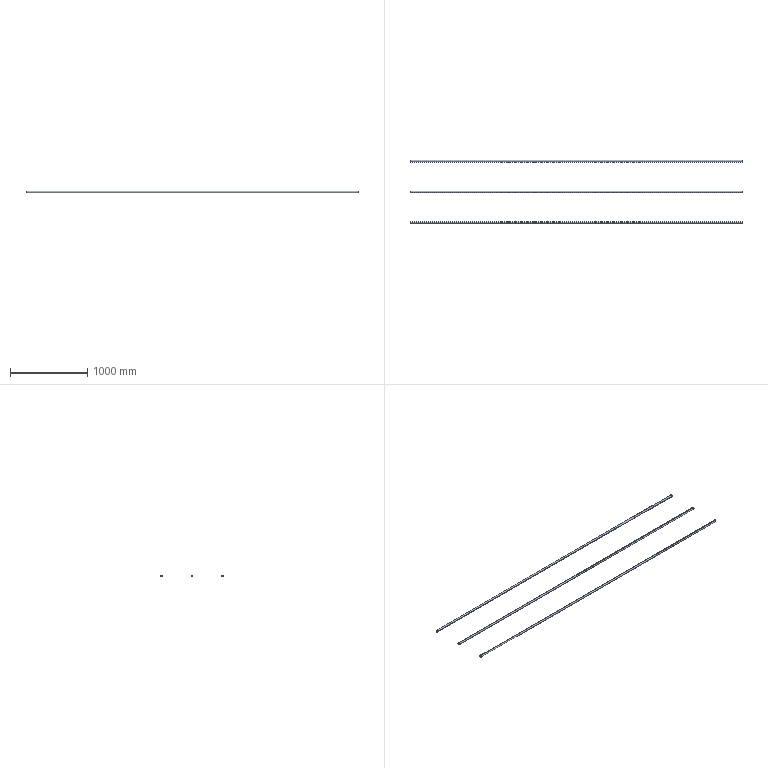Part | STEP file | 粉仓护栏栏杆1_Default<As Machined> | 3 solids | 18 faces | box 4305 x 825 x 25 mm | volume 1430222 mm3 | cylinder 12 | plane 6 | commonest cylinder face diameters 22 x6 25 x6
STEP:
#1=CARTESIAN_POINT('',(0.,0.,0.));
#2=DIRECTION('',(0.,0.,1.));
#3=DIRECTION('',(1.,0.,0.));
#4=AXIS2_PLACEMENT_3D('',#1,#2,#3);
#5=CARTESIAN_POINT('',(-4305.,0.,12.5));
#6=VERTEX_POINT('',#5);
#7=CARTESIAN_POINT('',(-4305.,0.,-12.5));
#8=VERTEX_POINT('',#7);
#9=CARTESIAN_POINT('',(-4305.,0.,0.));
#10=DIRECTION('',(-1.,0.,0.));
#11=DIRECTION('',(0.,-1.,0.));
#12=AXIS2_PLACEMENT_3D('',#9,#10,#11);
#13=CIRCLE('',#12,12.5);
#14=CARTESIAN_POINT('',(-4305.,0.,0.));
#15=DIRECTION('',(1.,0.,0.));
#16=DIRECTION('',(0.,0.,-1.));
#17=AXIS2_PLACEMENT_3D('',#14,#15,#16);
#18=CYLINDRICAL_SURFACE('',#17,12.5);
#19=CARTESIAN_POINT('',(4.712,0.));
#20=DIRECTION('',(-1.,0.));
#21=VECTOR('',#20,1.);
#22=LINE('',#19,#21);
#23=(GEOMETRIC_REPRESENTATION_CONTEXT(2)PARAMETRIC_REPRESENTATION_CONTEXT()REPRESENTATION_CONTEXT('',''));
#24=DEFINITIONAL_REPRESENTATION('',(#22),#23);
#25=PCURVE('',#18,#24);
#26=CARTESIAN_POINT('',(-4305.,0.,0.));
#27=DIRECTION('',(-1.,0.,0.));
#28=DIRECTION('',(0.,-1.,0.));
#29=AXIS2_PLACEMENT_3D('',#26,#27,#28);
#30=PLANE('',#29);
#31=CARTESIAN_POINT('',(0.,0.));
#32=DIRECTION('',(1.,0.));
#33=AXIS2_PLACEMENT_2D('',#31,#32);
#34=CIRCLE('',#33,12.5);
#35=(GEOMETRIC_REPRESENTATION_CONTEXT(2)PARAMETRIC_REPRESENTATION_CONTEXT()REPRESENTATION_CONTEXT('',''));
#36=DEFINITIONAL_REPRESENTATION('',(#34),#35);
#37=PCURVE('',#30,#36);
#38=SURFACE_CURVE('',#13,(#25,#37),.PCURVE_S1.);
#39=EDGE_CURVE('',#6,#8,#38,.T.);
#40=ORIENTED_EDGE('',*,*,#39,.F.);
#41=CARTESIAN_POINT('',(0.,0.,12.5));
#42=VERTEX_POINT('',#41);
#43=CARTESIAN_POINT('',(-4305.,0.,12.5));
#44=DIRECTION('',(1.,0.,0.));
#45=VECTOR('',#44,1.);
#46=LINE('',#43,#45);
#47=CARTESIAN_POINT('',(3.142,0.));
#48=DIRECTION('',(0.,1.));
#49=VECTOR('',#48,1.);
#50=LINE('',#47,#49);
#51=(GEOMETRIC_REPRESENTATION_CONTEXT(2)PARAMETRIC_REPRESENTATION_CONTEXT()REPRESENTATION_CONTEXT('',''));
#52=DEFINITIONAL_REPRESENTATION('',(#50),#51);
#53=PCURVE('',#18,#52);
#54=CARTESIAN_POINT('',(-4305.,0.,0.));
#55=DIRECTION('',(1.,0.,0.));
#56=DIRECTION('',(0.,0.,-1.));
#57=AXIS2_PLACEMENT_3D('',#54,#55,#56);
#58=CYLINDRICAL_SURFACE('',#57,12.5);
#59=CARTESIAN_POINT('',(3.142,0.));
#60=DIRECTION('',(0.,1.));
#61=VECTOR('',#60,1.);
#62=LINE('',#59,#61);
#63=(GEOMETRIC_REPRESENTATION_CONTEXT(2)PARAMETRIC_REPRESENTATION_CONTEXT()REPRESENTATION_CONTEXT('',''));
#64=DEFINITIONAL_REPRESENTATION('',(#62),#63);
#65=PCURVE('',#58,#64);
#66=SURFACE_CURVE('',#46,(#53,#65),.PCURVE_S1.);
#67=EDGE_CURVE('',#6,#42,#66,.T.);
#68=ORIENTED_EDGE('',*,*,#67,.T.);
#69=CARTESIAN_POINT('',(0.,0.,-12.5));
#70=VERTEX_POINT('',#69);
#71=CARTESIAN_POINT('',(0.,0.,0.));
#72=DIRECTION('',(-1.,0.,0.));
#73=DIRECTION('',(0.,-1.,0.));
#74=AXIS2_PLACEMENT_3D('',#71,#72,#73);
#75=CIRCLE('',#74,12.5);
#76=CARTESIAN_POINT('',(4.712,4305.));
#77=DIRECTION('',(-1.,0.));
#78=VECTOR('',#77,1.);
#79=LINE('',#76,#78);
#80=(GEOMETRIC_REPRESENTATION_CONTEXT(2)PARAMETRIC_REPRESENTATION_CONTEXT()REPRESENTATION_CONTEXT('',''));
#81=DEFINITIONAL_REPRESENTATION('',(#79),#80);
#82=PCURVE('',#18,#81);
#83=CARTESIAN_POINT('',(0.,0.,0.));
#84=DIRECTION('',(-1.,0.,0.));
#85=DIRECTION('',(0.,-1.,0.));
#86=AXIS2_PLACEMENT_3D('',#83,#84,#85);
#87=PLANE('',#86);
#88=CARTESIAN_POINT('',(0.,0.));
#89=DIRECTION('',(1.,0.));
#90=AXIS2_PLACEMENT_2D('',#88,#89);
#91=CIRCLE('',#90,12.5);
#92=(GEOMETRIC_REPRESENTATION_CONTEXT(2)PARAMETRIC_REPRESENTATION_CONTEXT()REPRESENTATION_CONTEXT('',''));
#93=DEFINITIONAL_REPRESENTATION('',(#91),#92);
#94=PCURVE('',#87,#93);
#95=SURFACE_CURVE('',#75,(#82,#94),.PCURVE_S1.);
#96=EDGE_CURVE('',#42,#70,#95,.T.);
#97=ORIENTED_EDGE('',*,*,#96,.T.);
#98=CARTESIAN_POINT('',(-4305.,0.,-12.5));
#99=DIRECTION('',(1.,0.,0.));
#100=VECTOR('',#99,1.);
#101=LINE('',#98,#100);
#102=CARTESIAN_POINT('',(0.,0.));
#103=DIRECTION('',(0.,1.));
#104=VECTOR('',#103,1.);
#105=LINE('',#102,#104);
#106=(GEOMETRIC_REPRESENTATION_CONTEXT(2)PARAMETRIC_REPRESENTATION_CONTEXT()REPRESENTATION_CONTEXT('',''));
#107=DEFINITIONAL_REPRESENTATION('',(#105),#106);
#108=PCURVE('',#18,#107);
#109=CARTESIAN_POINT('',(6.283,0.));
#110=DIRECTION('',(0.,1.));
#111=VECTOR('',#110,1.);
#112=LINE('',#109,#111);
#113=(GEOMETRIC_REPRESENTATION_CONTEXT(2)PARAMETRIC_REPRESENTATION_CONTEXT()REPRESENTATION_CONTEXT('',''));
#114=DEFINITIONAL_REPRESENTATION('',(#112),#113);
#115=PCURVE('',#58,#114);
#116=SURFACE_CURVE('',#101,(#108,#115),.PCURVE_S1.);
#117=EDGE_CURVE('',#8,#70,#116,.T.);
#118=ORIENTED_EDGE('',*,*,#117,.F.);
#119=EDGE_LOOP('',(#40,#68,#97,#118));
#120=FACE_BOUND('',#119,.T.);
#121=ADVANCED_FACE('',(#120),#18,.T.);
#122=CARTESIAN_POINT('',(-4305.,0.,-11.));
#123=VERTEX_POINT('',#122);
#124=CARTESIAN_POINT('',(0.,0.,-11.));
#125=VERTEX_POINT('',#124);
#126=CARTESIAN_POINT('',(-4305.,0.,-11.));
#127=DIRECTION('',(1.,0.,0.));
#128=VECTOR('',#127,1.);
#129=LINE('',#126,#128);
#130=CARTESIAN_POINT('',(-4305.,0.,0.));
#131=DIRECTION('',(1.,0.,0.));
#132=DIRECTION('',(0.,0.,-1.));
#133=AXIS2_PLACEMENT_3D('',#130,#131,#132);
#134=CYLINDRICAL_SURFACE('',#133,11.);
#135=CARTESIAN_POINT('',(6.283,0.));
#136=DIRECTION('',(0.,1.));
#137=VECTOR('',#136,1.);
#138=LINE('',#135,#137);
#139=(GEOMETRIC_REPRESENTATION_CONTEXT(2)PARAMETRIC_REPRESENTATION_CONTEXT()REPRESENTATION_CONTEXT('',''));
#140=DEFINITIONAL_REPRESENTATION('',(#138),#139);
#141=PCURVE('',#134,#140);
#142=CARTESIAN_POINT('',(-4305.,0.,0.));
#143=DIRECTION('',(1.,0.,0.));
#144=DIRECTION('',(0.,0.,-1.));
#145=AXIS2_PLACEMENT_3D('',#142,#143,#144);
#146=CYLINDRICAL_SURFACE('',#145,11.);
#147=CARTESIAN_POINT('',(0.,0.));
#148=DIRECTION('',(0.,1.));
#149=VECTOR('',#148,1.);
#150=LINE('',#147,#149);
#151=(GEOMETRIC_REPRESENTATION_CONTEXT(2)PARAMETRIC_REPRESENTATION_CONTEXT()REPRESENTATION_CONTEXT('',''));
#152=DEFINITIONAL_REPRESENTATION('',(#150),#151);
#153=PCURVE('',#146,#152);
#154=SURFACE_CURVE('',#129,(#141,#153),.PCURVE_S1.);
#155=EDGE_CURVE('',#123,#125,#154,.T.);
#156=ORIENTED_EDGE('',*,*,#155,.T.);
#157=CARTESIAN_POINT('',(0.,0.,11.));
#158=VERTEX_POINT('',#157);
#159=CARTESIAN_POINT('',(0.,0.,0.));
#160=DIRECTION('',(-1.,0.,0.));
#161=DIRECTION('',(0.,-1.,0.));
#162=AXIS2_PLACEMENT_3D('',#159,#160,#161);
#163=CIRCLE('',#162,11.);
#164=CARTESIAN_POINT('',(10.996,4305.));
#165=DIRECTION('',(-1.,0.));
#166=VECTOR('',#165,1.);
#167=LINE('',#164,#166);
#168=(GEOMETRIC_REPRESENTATION_CONTEXT(2)PARAMETRIC_REPRESENTATION_CONTEXT()REPRESENTATION_CONTEXT('',''));
#169=DEFINITIONAL_REPRESENTATION('',(#167),#168);
#170=PCURVE('',#134,#169);
#171=CARTESIAN_POINT('',(0.,0.));
#172=DIRECTION('',(1.,0.));
#173=AXIS2_PLACEMENT_2D('',#171,#172);
#174=CIRCLE('',#173,11.);
#175=(GEOMETRIC_REPRESENTATION_CONTEXT(2)PARAMETRIC_REPRESENTATION_CONTEXT()REPRESENTATION_CONTEXT('',''));
#176=DEFINITIONAL_REPRESENTATION('',(#174),#175);
#177=PCURVE('',#87,#176);
#178=SURFACE_CURVE('',#163,(#170,#177),.PCURVE_S1.);
#179=EDGE_CURVE('',#125,#158,#178,.T.);
#180=ORIENTED_EDGE('',*,*,#179,.T.);
#181=CARTESIAN_POINT('',(-4305.,0.,11.));
#182=VERTEX_POINT('',#181);
#183=CARTESIAN_POINT('',(-4305.,0.,11.));
#184=DIRECTION('',(1.,0.,0.));
#185=VECTOR('',#184,1.);
#186=LINE('',#183,#185);
#187=CARTESIAN_POINT('',(3.142,0.));
#188=DIRECTION('',(0.,1.));
#189=VECTOR('',#188,1.);
#190=LINE('',#187,#189);
#191=(GEOMETRIC_REPRESENTATION_CONTEXT(2)PARAMETRIC_REPRESENTATION_CONTEXT()REPRESENTATION_CONTEXT('',''));
#192=DEFINITIONAL_REPRESENTATION('',(#190),#191);
#193=PCURVE('',#134,#192);
#194=CARTESIAN_POINT('',(3.142,0.));
#195=DIRECTION('',(0.,1.));
#196=VECTOR('',#195,1.);
#197=LINE('',#194,#196);
#198=(GEOMETRIC_REPRESENTATION_CONTEXT(2)PARAMETRIC_REPRESENTATION_CONTEXT()REPRESENTATION_CONTEXT('',''));
#199=DEFINITIONAL_REPRESENTATION('',(#197),#198);
#200=PCURVE('',#146,#199);
#201=SURFACE_CURVE('',#186,(#193,#200),.PCURVE_S1.);
#202=EDGE_CURVE('',#182,#158,#201,.T.);
#203=ORIENTED_EDGE('',*,*,#202,.F.);
#204=CARTESIAN_POINT('',(-4305.,0.,0.));
#205=DIRECTION('',(-1.,0.,0.));
#206=DIRECTION('',(0.,-1.,0.));
#207=AXIS2_PLACEMENT_3D('',#204,#205,#206);
#208=CIRCLE('',#207,11.);
#209=CARTESIAN_POINT('',(10.996,0.));
#210=DIRECTION('',(-1.,0.));
#211=VECTOR('',#210,1.);
#212=LINE('',#209,#211);
#213=(GEOMETRIC_REPRESENTATION_CONTEXT(2)PARAMETRIC_REPRESENTATION_CONTEXT()REPRESENTATION_CONTEXT('',''));
#214=DEFINITIONAL_REPRESENTATION('',(#212),#213);
#215=PCURVE('',#134,#214);
#216=CARTESIAN_POINT('',(0.,0.));
#217=DIRECTION('',(1.,0.));
#218=AXIS2_PLACEMENT_2D('',#216,#217);
#219=CIRCLE('',#218,11.);
#220=(GEOMETRIC_REPRESENTATION_CONTEXT(2)PARAMETRIC_REPRESENTATION_CONTEXT()REPRESENTATION_CONTEXT('',''));
#221=DEFINITIONAL_REPRESENTATION('',(#219),#220);
#222=PCURVE('',#30,#221);
#223=SURFACE_CURVE('',#208,(#215,#222),.PCURVE_S1.);
#224=EDGE_CURVE('',#123,#182,#223,.T.);
#225=ORIENTED_EDGE('',*,*,#224,.F.);
#226=EDGE_LOOP('',(#156,#180,#203,#225));
#227=FACE_BOUND('',#226,.F.);
#228=ADVANCED_FACE('',(#227),#134,.F.);
#229=CARTESIAN_POINT('',(0.,0.,0.));
#230=DIRECTION('',(-1.,0.,0.));
#231=DIRECTION('',(0.,-1.,0.));
#232=AXIS2_PLACEMENT_3D('',#229,#230,#231);
#233=CIRCLE('',#232,11.);
#234=CARTESIAN_POINT('',(4.712,4305.));
#235=DIRECTION('',(-1.,0.));
#236=VECTOR('',#235,1.);
#237=LINE('',#234,#236);
#238=(GEOMETRIC_REPRESENTATION_CONTEXT(2)PARAMETRIC_REPRESENTATION_CONTEXT()REPRESENTATION_CONTEXT('',''));
#239=DEFINITIONAL_REPRESENTATION('',(#237),#238);
#240=PCURVE('',#146,#239);
#241=CARTESIAN_POINT('',(0.,0.));
#242=DIRECTION('',(1.,0.));
#243=AXIS2_PLACEMENT_2D('',#241,#242);
#244=CIRCLE('',#243,11.);
#245=(GEOMETRIC_REPRESENTATION_CONTEXT(2)PARAMETRIC_REPRESENTATION_CONTEXT()REPRESENTATION_CONTEXT('',''));
#246=DEFINITIONAL_REPRESENTATION('',(#244),#245);
#247=PCURVE('',#87,#246);
#248=SURFACE_CURVE('',#233,(#240,#247),.PCURVE_S1.);
#249=EDGE_CURVE('',#158,#125,#248,.T.);
#250=ORIENTED_EDGE('',*,*,#249,.T.);
#251=ORIENTED_EDGE('',*,*,#155,.F.);
#252=CARTESIAN_POINT('',(-4305.,0.,0.));
#253=DIRECTION('',(-1.,0.,0.));
#254=DIRECTION('',(0.,-1.,0.));
#255=AXIS2_PLACEMENT_3D('',#252,#253,#254);
#256=CIRCLE('',#255,11.);
#257=CARTESIAN_POINT('',(4.712,0.));
#258=DIRECTION('',(-1.,0.));
#259=VECTOR('',#258,1.);
#260=LINE('',#257,#259);
#261=(GEOMETRIC_REPRESENTATION_CONTEXT(2)PARAMETRIC_REPRESENTATION_CONTEXT()REPRESENTATION_CONTEXT('',''));
#262=DEFINITIONAL_REPRESENTATION('',(#260),#261);
#263=PCURVE('',#146,#262);
#264=CARTESIAN_POINT('',(0.,0.));
#265=DIRECTION('',(1.,0.));
#266=AXIS2_PLACEMENT_2D('',#264,#265);
#267=CIRCLE('',#266,11.);
#268=(GEOMETRIC_REPRESENTATION_CONTEXT(2)PARAMETRIC_REPRESENTATION_CONTEXT()REPRESENTATION_CONTEXT('',''));
#269=DEFINITIONAL_REPRESENTATION('',(#267),#268);
#270=PCURVE('',#30,#269);
#271=SURFACE_CURVE('',#256,(#263,#270),.PCURVE_S1.);
#272=EDGE_CURVE('',#182,#123,#271,.T.);
#273=ORIENTED_EDGE('',*,*,#272,.F.);
#274=ORIENTED_EDGE('',*,*,#202,.T.);
#275=EDGE_LOOP('',(#250,#251,#273,#274));
#276=FACE_BOUND('',#275,.F.);
#277=ADVANCED_FACE('',(#276),#146,.F.);
#278=ORIENTED_EDGE('',*,*,#67,.F.);
#279=CARTESIAN_POINT('',(-4305.,0.,0.));
#280=DIRECTION('',(-1.,0.,0.));
#281=DIRECTION('',(0.,-1.,0.));
#282=AXIS2_PLACEMENT_3D('',#279,#280,#281);
#283=CIRCLE('',#282,12.5);
#284=CARTESIAN_POINT('',(10.996,0.));
#285=DIRECTION('',(-1.,0.));
#286=VECTOR('',#285,1.);
#287=LINE('',#284,#286);
#288=(GEOMETRIC_REPRESENTATION_CONTEXT(2)PARAMETRIC_REPRESENTATION_CONTEXT()REPRESENTATION_CONTEXT('',''));
#289=DEFINITIONAL_REPRESENTATION('',(#287),#288);
#290=PCURVE('',#58,#289);
#291=CARTESIAN_POINT('',(0.,0.));
#292=DIRECTION('',(1.,0.));
#293=AXIS2_PLACEMENT_2D('',#291,#292);
#294=CIRCLE('',#293,12.5);
#295=(GEOMETRIC_REPRESENTATION_CONTEXT(2)PARAMETRIC_REPRESENTATION_CONTEXT()REPRESENTATION_CONTEXT('',''));
#296=DEFINITIONAL_REPRESENTATION('',(#294),#295);
#297=PCURVE('',#30,#296);
#298=SURFACE_CURVE('',#283,(#290,#297),.PCURVE_S1.);
#299=EDGE_CURVE('',#8,#6,#298,.T.);
#300=ORIENTED_EDGE('',*,*,#299,.F.);
#301=ORIENTED_EDGE('',*,*,#117,.T.);
#302=CARTESIAN_POINT('',(0.,0.,0.));
#303=DIRECTION('',(-1.,0.,0.));
#304=DIRECTION('',(0.,-1.,0.));
#305=AXIS2_PLACEMENT_3D('',#302,#303,#304);
#306=CIRCLE('',#305,12.5);
#307=CARTESIAN_POINT('',(10.996,4305.));
#308=DIRECTION('',(-1.,0.));
#309=VECTOR('',#308,1.);
#310=LINE('',#307,#309);
#311=(GEOMETRIC_REPRESENTATION_CONTEXT(2)PARAMETRIC_REPRESENTATION_CONTEXT()REPRESENTATION_CONTEXT('',''));
#312=DEFINITIONAL_REPRESENTATION('',(#310),#311);
#313=PCURVE('',#58,#312);
#314=CARTESIAN_POINT('',(0.,0.));
#315=DIRECTION('',(1.,0.));
#316=AXIS2_PLACEMENT_2D('',#314,#315);
#317=CIRCLE('',#316,12.5);
#318=(GEOMETRIC_REPRESENTATION_CONTEXT(2)PARAMETRIC_REPRESENTATION_CONTEXT()REPRESENTATION_CONTEXT('',''));
#319=DEFINITIONAL_REPRESENTATION('',(#317),#318);
#320=PCURVE('',#87,#319);
#321=SURFACE_CURVE('',#306,(#313,#320),.PCURVE_S1.);
#322=EDGE_CURVE('',#70,#42,#321,.T.);
#323=ORIENTED_EDGE('',*,*,#322,.T.);
#324=EDGE_LOOP('',(#278,#300,#301,#323));
#325=FACE_BOUND('',#324,.T.);
#326=ADVANCED_FACE('',(#325),#58,.T.);
#327=ORIENTED_EDGE('',*,*,#224,.F.);
#328=ORIENTED_EDGE('',*,*,#272,.F.);
#329=EDGE_LOOP('',(#327,#328));
#330=FACE_BOUND('',#329,.T.);
#331=ORIENTED_EDGE('',*,*,#299,.T.);
#332=ORIENTED_EDGE('',*,*,#39,.T.);
#333=EDGE_LOOP('',(#331,#332));
#334=FACE_BOUND('',#333,.T.);
#335=ADVANCED_FACE('',(#330,#334),#30,.T.);
#336=ORIENTED_EDGE('',*,*,#179,.T.);
#337=ORIENTED_EDGE('',*,*,#249,.T.);
#338=EDGE_LOOP('',(#336,#337));
#339=FACE_BOUND('',#338,.T.);
#340=ORIENTED_EDGE('',*,*,#322,.F.);
#341=ORIENTED_EDGE('',*,*,#96,.F.);
#342=EDGE_LOOP('',(#340,#341));
#343=FACE_BOUND('',#342,.T.);
#344=ADVANCED_FACE('',(#339,#343),#87,.F.);
#345=CLOSED_SHELL('',(#121,#228,#277,#326,#335,#344));
#346=MANIFOLD_SOLID_BREP('',#345);
#347=CARTESIAN_POINT('',(-4305.,787.5,0.));
#348=VERTEX_POINT('',#347);
#349=CARTESIAN_POINT('',(-4305.,812.5,0.));
#350=VERTEX_POINT('',#349);
#351=CARTESIAN_POINT('',(-4305.,800.,0.));
#352=DIRECTION('',(-1.,0.,0.));
#353=DIRECTION('',(0.,-1.,0.));
#354=AXIS2_PLACEMENT_3D('',#351,#352,#353);
#355=CIRCLE('',#354,12.5);
#356=CARTESIAN_POINT('',(-4305.,800.,0.));
#357=DIRECTION('',(1.,0.,0.));
#358=DIRECTION('',(0.,1.,0.));
#359=AXIS2_PLACEMENT_3D('',#356,#357,#358);
#360=CYLINDRICAL_SURFACE('',#359,12.5);
#361=CARTESIAN_POINT('',(3.142,0.));
#362=DIRECTION('',(-1.,0.));
#363=VECTOR('',#362,1.);
#364=LINE('',#361,#363);
#365=(GEOMETRIC_REPRESENTATION_CONTEXT(2)PARAMETRIC_REPRESENTATION_CONTEXT()REPRESENTATION_CONTEXT('',''));
#366=DEFINITIONAL_REPRESENTATION('',(#364),#365);
#367=PCURVE('',#360,#366);
#368=CARTESIAN_POINT('',(-4305.,800.,0.));
#369=DIRECTION('',(-1.,0.,0.));
#370=DIRECTION('',(0.,-1.,0.));
#371=AXIS2_PLACEMENT_3D('',#368,#369,#370);
#372=PLANE('',#371);
#373=CARTESIAN_POINT('',(0.,0.));
#374=DIRECTION('',(1.,0.));
#375=AXIS2_PLACEMENT_2D('',#373,#374);
#376=CIRCLE('',#375,12.5);
#377=(GEOMETRIC_REPRESENTATION_CONTEXT(2)PARAMETRIC_REPRESENTATION_CONTEXT()REPRESENTATION_CONTEXT('',''));
#378=DEFINITIONAL_REPRESENTATION('',(#376),#377);
#379=PCURVE('',#372,#378);
#380=SURFACE_CURVE('',#355,(#367,#379),.PCURVE_S1.);
#381=EDGE_CURVE('',#348,#350,#380,.T.);
#382=ORIENTED_EDGE('',*,*,#381,.F.);
#383=CARTESIAN_POINT('',(0.,787.5,0.));
#384=VERTEX_POINT('',#383);
#385=CARTESIAN_POINT('',(-4305.,787.5,0.));
#386=DIRECTION('',(1.,0.,0.));
#387=VECTOR('',#386,1.);
#388=LINE('',#385,#387);
#389=CARTESIAN_POINT('',(3.142,0.));
#390=DIRECTION('',(0.,1.));
#391=VECTOR('',#390,1.);
#392=LINE('',#389,#391);
#393=(GEOMETRIC_REPRESENTATION_CONTEXT(2)PARAMETRIC_REPRESENTATION_CONTEXT()REPRESENTATION_CONTEXT('',''));
#394=DEFINITIONAL_REPRESENTATION('',(#392),#393);
#395=PCURVE('',#360,#394);
#396=CARTESIAN_POINT('',(-4305.,800.,0.));
#397=DIRECTION('',(1.,0.,0.));
#398=DIRECTION('',(0.,1.,0.));
#399=AXIS2_PLACEMENT_3D('',#396,#397,#398);
#400=CYLINDRICAL_SURFACE('',#399,12.5);
#401=CARTESIAN_POINT('',(3.142,0.));
#402=DIRECTION('',(0.,1.));
#403=VECTOR('',#402,1.);
#404=LINE('',#401,#403);
#405=(GEOMETRIC_REPRESENTATION_CONTEXT(2)PARAMETRIC_REPRESENTATION_CONTEXT()REPRESENTATION_CONTEXT('',''));
#406=DEFINITIONAL_REPRESENTATION('',(#404),#405);
#407=PCURVE('',#400,#406);
#408=SURFACE_CURVE('',#388,(#395,#407),.PCURVE_S1.);
#409=EDGE_CURVE('',#348,#384,#408,.T.);
#410=ORIENTED_EDGE('',*,*,#409,.T.);
#411=CARTESIAN_POINT('',(0.,812.5,0.));
#412=VERTEX_POINT('',#411);
#413=CARTESIAN_POINT('',(0.,800.,0.));
#414=DIRECTION('',(-1.,0.,0.));
#415=DIRECTION('',(0.,-1.,0.));
#416=AXIS2_PLACEMENT_3D('',#413,#414,#415);
#417=CIRCLE('',#416,12.5);
#418=CARTESIAN_POINT('',(3.142,4305.));
#419=DIRECTION('',(-1.,0.));
#420=VECTOR('',#419,1.);
#421=LINE('',#418,#420);
#422=(GEOMETRIC_REPRESENTATION_CONTEXT(2)PARAMETRIC_REPRESENTATION_CONTEXT()REPRESENTATION_CONTEXT('',''));
#423=DEFINITIONAL_REPRESENTATION('',(#421),#422);
#424=PCURVE('',#360,#423);
#425=CARTESIAN_POINT('',(0.,800.,0.));
#426=DIRECTION('',(-1.,0.,0.));
#427=DIRECTION('',(0.,-1.,0.));
#428=AXIS2_PLACEMENT_3D('',#425,#426,#427);
#429=PLANE('',#428);
#430=CARTESIAN_POINT('',(0.,0.));
#431=DIRECTION('',(1.,0.));
#432=AXIS2_PLACEMENT_2D('',#430,#431);
#433=CIRCLE('',#432,12.5);
#434=(GEOMETRIC_REPRESENTATION_CONTEXT(2)PARAMETRIC_REPRESENTATION_CONTEXT()REPRESENTATION_CONTEXT('',''));
#435=DEFINITIONAL_REPRESENTATION('',(#433),#434);
#436=PCURVE('',#429,#435);
#437=SURFACE_CURVE('',#417,(#424,#436),.PCURVE_S1.);
#438=EDGE_CURVE('',#384,#412,#437,.T.);
#439=ORIENTED_EDGE('',*,*,#438,.T.);
#440=CARTESIAN_POINT('',(-4305.,812.5,0.));
#441=DIRECTION('',(1.,0.,0.));
#442=VECTOR('',#441,1.);
#443=LINE('',#440,#442);
#444=CARTESIAN_POINT('',(0.,0.));
#445=DIRECTION('',(0.,1.));
#446=VECTOR('',#445,1.);
#447=LINE('',#444,#446);
#448=(GEOMETRIC_REPRESENTATION_CONTEXT(2)PARAMETRIC_REPRESENTATION_CONTEXT()REPRESENTATION_CONTEXT('',''));
#449=DEFINITIONAL_REPRESENTATION('',(#447),#448);
#450=PCURVE('',#360,#449);
#451=CARTESIAN_POINT('',(6.283,0.));
#452=DIRECTION('',(0.,1.));
#453=VECTOR('',#452,1.);
#454=LINE('',#451,#453);
#455=(GEOMETRIC_REPRESENTATION_CONTEXT(2)PARAMETRIC_REPRESENTATION_CONTEXT()REPRESENTATION_CONTEXT('',''));
#456=DEFINITIONAL_REPRESENTATION('',(#454),#455);
#457=PCURVE('',#400,#456);
#458=SURFACE_CURVE('',#443,(#450,#457),.PCURVE_S1.);
#459=EDGE_CURVE('',#350,#412,#458,.T.);
#460=ORIENTED_EDGE('',*,*,#459,.F.);
#461=EDGE_LOOP('',(#382,#410,#439,#460));
#462=FACE_BOUND('',#461,.T.);
#463=ADVANCED_FACE('',(#462),#360,.T.);
#464=CARTESIAN_POINT('',(-4305.,811.,0.));
#465=VERTEX_POINT('',#464);
#466=CARTESIAN_POINT('',(0.,811.,0.));
#467=VERTEX_POINT('',#466);
#468=CARTESIAN_POINT('',(-4305.,811.,0.));
#469=DIRECTION('',(1.,0.,0.));
#470=VECTOR('',#469,1.);
#471=LINE('',#468,#470);
#472=CARTESIAN_POINT('',(-4305.,800.,0.));
#473=DIRECTION('',(1.,0.,0.));
#474=DIRECTION('',(0.,1.,0.));
#475=AXIS2_PLACEMENT_3D('',#472,#473,#474);
#476=CYLINDRICAL_SURFACE('',#475,11.);
#477=CARTESIAN_POINT('',(6.283,0.));
#478=DIRECTION('',(0.,1.));
#479=VECTOR('',#478,1.);
#480=LINE('',#477,#479);
#481=(GEOMETRIC_REPRESENTATION_CONTEXT(2)PARAMETRIC_REPRESENTATION_CONTEXT()REPRESENTATION_CONTEXT('',''));
#482=DEFINITIONAL_REPRESENTATION('',(#480),#481);
#483=PCURVE('',#476,#482);
#484=CARTESIAN_POINT('',(-4305.,800.,0.));
#485=DIRECTION('',(1.,0.,0.));
#486=DIRECTION('',(0.,1.,0.));
#487=AXIS2_PLACEMENT_3D('',#484,#485,#486);
#488=CYLINDRICAL_SURFACE('',#487,11.);
#489=CARTESIAN_POINT('',(0.,0.));
#490=DIRECTION('',(0.,1.));
#491=VECTOR('',#490,1.);
#492=LINE('',#489,#491);
#493=(GEOMETRIC_REPRESENTATION_CONTEXT(2)PARAMETRIC_REPRESENTATION_CONTEXT()REPRESENTATION_CONTEXT('',''));
#494=DEFINITIONAL_REPRESENTATION('',(#492),#493);
#495=PCURVE('',#488,#494);
#496=SURFACE_CURVE('',#471,(#483,#495),.PCURVE_S1.);
#497=EDGE_CURVE('',#465,#467,#496,.T.);
#498=ORIENTED_EDGE('',*,*,#497,.T.);
#499=CARTESIAN_POINT('',(0.,789.,0.));
#500=VERTEX_POINT('',#499);
#501=CARTESIAN_POINT('',(0.,800.,0.));
#502=DIRECTION('',(-1.,0.,0.));
#503=DIRECTION('',(0.,-1.,0.));
#504=AXIS2_PLACEMENT_3D('',#501,#502,#503);
#505=CIRCLE('',#504,11.);
#506=CARTESIAN_POINT('',(9.425,4305.));
#507=DIRECTION('',(-1.,0.));
#508=VECTOR('',#507,1.);
#509=LINE('',#506,#508);
#510=(GEOMETRIC_REPRESENTATION_CONTEXT(2)PARAMETRIC_REPRESENTATION_CONTEXT()REPRESENTATION_CONTEXT('',''));
#511=DEFINITIONAL_REPRESENTATION('',(#509),#510);
#512=PCURVE('',#476,#511);
#513=CARTESIAN_POINT('',(0.,0.));
#514=DIRECTION('',(1.,0.));
#515=AXIS2_PLACEMENT_2D('',#513,#514);
#516=CIRCLE('',#515,11.);
#517=(GEOMETRIC_REPRESENTATION_CONTEXT(2)PARAMETRIC_REPRESENTATION_CONTEXT()REPRESENTATION_CONTEXT('',''));
#518=DEFINITIONAL_REPRESENTATION('',(#516),#517);
#519=PCURVE('',#429,#518);
#520=SURFACE_CURVE('',#505,(#512,#519),.PCURVE_S1.);
#521=EDGE_CURVE('',#467,#500,#520,.T.);
#522=ORIENTED_EDGE('',*,*,#521,.T.);
#523=CARTESIAN_POINT('',(-4305.,789.,0.));
#524=VERTEX_POINT('',#523);
#525=CARTESIAN_POINT('',(-4305.,789.,0.));
#526=DIRECTION('',(1.,0.,0.));
#527=VECTOR('',#526,1.);
#528=LINE('',#525,#527);
#529=CARTESIAN_POINT('',(3.142,0.));
#530=DIRECTION('',(0.,1.));
#531=VECTOR('',#530,1.);
#532=LINE('',#529,#531);
#533=(GEOMETRIC_REPRESENTATION_CONTEXT(2)PARAMETRIC_REPRESENTATION_CONTEXT()REPRESENTATION_CONTEXT('',''));
#534=DEFINITIONAL_REPRESENTATION('',(#532),#533);
#535=PCURVE('',#476,#534);
#536=CARTESIAN_POINT('',(3.142,0.));
#537=DIRECTION('',(0.,1.));
#538=VECTOR('',#537,1.);
#539=LINE('',#536,#538);
#540=(GEOMETRIC_REPRESENTATION_CONTEXT(2)PARAMETRIC_REPRESENTATION_CONTEXT()REPRESENTATION_CONTEXT('',''));
#541=DEFINITIONAL_REPRESENTATION('',(#539),#540);
#542=PCURVE('',#488,#541);
#543=SURFACE_CURVE('',#528,(#535,#542),.PCURVE_S1.);
#544=EDGE_CURVE('',#524,#500,#543,.T.);
#545=ORIENTED_EDGE('',*,*,#544,.F.);
#546=CARTESIAN_POINT('',(-4305.,800.,0.));
#547=DIRECTION('',(-1.,0.,0.));
#548=DIRECTION('',(0.,-1.,0.));
#549=AXIS2_PLACEMENT_3D('',#546,#547,#548);
#550=CIRCLE('',#549,11.);
#551=CARTESIAN_POINT('',(9.425,0.));
#552=DIRECTION('',(-1.,0.));
#553=VECTOR('',#552,1.);
#554=LINE('',#551,#553);
#555=(GEOMETRIC_REPRESENTATION_CONTEXT(2)PARAMETRIC_REPRESENTATION_CONTEXT()REPRESENTATION_CONTEXT('',''));
#556=DEFINITIONAL_REPRESENTATION('',(#554),#555);
#557=PCURVE('',#476,#556);
#558=CARTESIAN_POINT('',(0.,0.));
#559=DIRECTION('',(1.,0.));
#560=AXIS2_PLACEMENT_2D('',#558,#559);
#561=CIRCLE('',#560,11.);
#562=(GEOMETRIC_REPRESENTATION_CONTEXT(2)PARAMETRIC_REPRESENTATION_CONTEXT()REPRESENTATION_CONTEXT('',''));
#563=DEFINITIONAL_REPRESENTATION('',(#561),#562);
#564=PCURVE('',#372,#563);
#565=SURFACE_CURVE('',#550,(#557,#564),.PCURVE_S1.);
#566=EDGE_CURVE('',#465,#524,#565,.T.);
#567=ORIENTED_EDGE('',*,*,#566,.F.);
#568=EDGE_LOOP('',(#498,#522,#545,#567));
#569=FACE_BOUND('',#568,.F.);
#570=ADVANCED_FACE('',(#569),#476,.F.);
#571=CARTESIAN_POINT('',(0.,800.,0.));
#572=DIRECTION('',(-1.,0.,0.));
#573=DIRECTION('',(0.,-1.,0.));
#574=AXIS2_PLACEMENT_3D('',#571,#572,#573);
#575=CIRCLE('',#574,11.);
#576=CARTESIAN_POINT('',(3.142,4305.));
#577=DIRECTION('',(-1.,0.));
#578=VECTOR('',#577,1.);
#579=LINE('',#576,#578);
#580=(GEOMETRIC_REPRESENTATION_CONTEXT(2)PARAMETRIC_REPRESENTATION_CONTEXT()REPRESENTATION_CONTEXT('',''));
#581=DEFINITIONAL_REPRESENTATION('',(#579),#580);
#582=PCURVE('',#488,#581);
#583=CARTESIAN_POINT('',(0.,0.));
#584=DIRECTION('',(1.,0.));
#585=AXIS2_PLACEMENT_2D('',#583,#584);
#586=CIRCLE('',#585,11.);
#587=(GEOMETRIC_REPRESENTATION_CONTEXT(2)PARAMETRIC_REPRESENTATION_CONTEXT()REPRESENTATION_CONTEXT('',''));
#588=DEFINITIONAL_REPRESENTATION('',(#586),#587);
#589=PCURVE('',#429,#588);
#590=SURFACE_CURVE('',#575,(#582,#589),.PCURVE_S1.);
#591=EDGE_CURVE('',#500,#467,#590,.T.);
#592=ORIENTED_EDGE('',*,*,#591,.T.);
#593=ORIENTED_EDGE('',*,*,#497,.F.);
#594=CARTESIAN_POINT('',(-4305.,800.,0.));
#595=DIRECTION('',(-1.,0.,0.));
#596=DIRECTION('',(0.,-1.,0.));
#597=AXIS2_PLACEMENT_3D('',#594,#595,#596);
#598=CIRCLE('',#597,11.);
#599=CARTESIAN_POINT('',(3.142,0.));
#600=DIRECTION('',(-1.,0.));
#601=VECTOR('',#600,1.);
#602=LINE('',#599,#601);
#603=(GEOMETRIC_REPRESENTATION_CONTEXT(2)PARAMETRIC_REPRESENTATION_CONTEXT()REPRESENTATION_CONTEXT('',''));
#604=DEFINITIONAL_REPRESENTATION('',(#602),#603);
#605=PCURVE('',#488,#604);
#606=CARTESIAN_POINT('',(0.,0.));
#607=DIRECTION('',(1.,0.));
#608=AXIS2_PLACEMENT_2D('',#606,#607);
#609=CIRCLE('',#608,11.);
#610=(GEOMETRIC_REPRESENTATION_CONTEXT(2)PARAMETRIC_REPRESENTATION_CONTEXT()REPRESENTATION_CONTEXT('',''));
#611=DEFINITIONAL_REPRESENTATION('',(#609),#610);
#612=PCURVE('',#372,#611);
#613=SURFACE_CURVE('',#598,(#605,#612),.PCURVE_S1.);
#614=EDGE_CURVE('',#524,#465,#613,.T.);
#615=ORIENTED_EDGE('',*,*,#614,.F.);
#616=ORIENTED_EDGE('',*,*,#544,.T.);
#617=EDGE_LOOP('',(#592,#593,#615,#616));
#618=FACE_BOUND('',#617,.F.);
#619=ADVANCED_FACE('',(#618),#488,.F.);
#620=ORIENTED_EDGE('',*,*,#409,.F.);
#621=CARTESIAN_POINT('',(-4305.,800.,0.));
#622=DIRECTION('',(-1.,0.,0.));
#623=DIRECTION('',(0.,-1.,0.));
#624=AXIS2_PLACEMENT_3D('',#621,#622,#623);
#625=CIRCLE('',#624,12.5);
#626=CARTESIAN_POINT('',(9.425,0.));
#627=DIRECTION('',(-1.,0.));
#628=VECTOR('',#627,1.);
#629=LINE('',#626,#628);
#630=(GEOMETRIC_REPRESENTATION_CONTEXT(2)PARAMETRIC_REPRESENTATION_CONTEXT()REPRESENTATION_CONTEXT('',''));
#631=DEFINITIONAL_REPRESENTATION('',(#629),#630);
#632=PCURVE('',#400,#631);
#633=CARTESIAN_POINT('',(0.,0.));
#634=DIRECTION('',(1.,0.));
#635=AXIS2_PLACEMENT_2D('',#633,#634);
#636=CIRCLE('',#635,12.5);
#637=(GEOMETRIC_REPRESENTATION_CONTEXT(2)PARAMETRIC_REPRESENTATION_CONTEXT()REPRESENTATION_CONTEXT('',''));
#638=DEFINITIONAL_REPRESENTATION('',(#636),#637);
#639=PCURVE('',#372,#638);
#640=SURFACE_CURVE('',#625,(#632,#639),.PCURVE_S1.);
#641=EDGE_CURVE('',#350,#348,#640,.T.);
#642=ORIENTED_EDGE('',*,*,#641,.F.);
#643=ORIENTED_EDGE('',*,*,#459,.T.);
#644=CARTESIAN_POINT('',(0.,800.,0.));
#645=DIRECTION('',(-1.,0.,0.));
#646=DIRECTION('',(0.,-1.,0.));
#647=AXIS2_PLACEMENT_3D('',#644,#645,#646);
#648=CIRCLE('',#647,12.5);
#649=CARTESIAN_POINT('',(9.425,4305.));
#650=DIRECTION('',(-1.,0.));
#651=VECTOR('',#650,1.);
#652=LINE('',#649,#651);
#653=(GEOMETRIC_REPRESENTATION_CONTEXT(2)PARAMETRIC_REPRESENTATION_CONTEXT()REPRESENTATION_CONTEXT('',''));
#654=DEFINITIONAL_REPRESENTATION('',(#652),#653);
#655=PCURVE('',#400,#654);
#656=CARTESIAN_POINT('',(0.,0.));
#657=DIRECTION('',(1.,0.));
#658=AXIS2_PLACEMENT_2D('',#656,#657);
#659=CIRCLE('',#658,12.5);
#660=(GEOMETRIC_REPRESENTATION_CONTEXT(2)PARAMETRIC_REPRESENTATION_CONTEXT()REPRESENTATION_CONTEXT('',''));
#661=DEFINITIONAL_REPRESENTATION('',(#659),#660);
#662=PCURVE('',#429,#661);
#663=SURFACE_CURVE('',#648,(#655,#662),.PCURVE_S1.);
#664=EDGE_CURVE('',#412,#384,#663,.T.);
#665=ORIENTED_EDGE('',*,*,#664,.T.);
#666=EDGE_LOOP('',(#620,#642,#643,#665));
#667=FACE_BOUND('',#666,.T.);
#668=ADVANCED_FACE('',(#667),#400,.T.);
#669=ORIENTED_EDGE('',*,*,#566,.F.);
#670=ORIENTED_EDGE('',*,*,#614,.F.);
#671=EDGE_LOOP('',(#669,#670));
#672=FACE_BOUND('',#671,.T.);
#673=ORIENTED_EDGE('',*,*,#641,.T.);
#674=ORIENTED_EDGE('',*,*,#381,.T.);
#675=EDGE_LOOP('',(#673,#674));
#676=FACE_BOUND('',#675,.T.);
#677=ADVANCED_FACE('',(#672,#676),#372,.T.);
#678=ORIENTED_EDGE('',*,*,#521,.T.);
#679=ORIENTED_EDGE('',*,*,#591,.T.);
#680=EDGE_LOOP('',(#678,#679));
#681=FACE_BOUND('',#680,.T.);
#682=ORIENTED_EDGE('',*,*,#664,.F.);
#683=ORIENTED_EDGE('',*,*,#438,.F.);
#684=EDGE_LOOP('',(#682,#683));
#685=FACE_BOUND('',#684,.T.);
#686=ADVANCED_FACE('',(#681,#685),#429,.F.);
#687=CLOSED_SHELL('',(#463,#570,#619,#668,#677,#686));
#688=MANIFOLD_SOLID_BREP('',#687);
#689=CARTESIAN_POINT('',(0.,400.,-12.5));
#690=VERTEX_POINT('',#689);
#691=CARTESIAN_POINT('',(0.,400.,12.5));
#692=VERTEX_POINT('',#691);
#693=CARTESIAN_POINT('',(0.,400.,0.));
#694=DIRECTION('',(1.,0.,0.));
#695=DIRECTION('',(0.,1.,0.));
#696=AXIS2_PLACEMENT_3D('',#693,#694,#695);
#697=CIRCLE('',#696,12.5);
#698=CARTESIAN_POINT('',(0.,400.,0.));
#699=DIRECTION('',(-1.,0.,0.));
#700=DIRECTION('',(0.,0.,1.));
#701=AXIS2_PLACEMENT_3D('',#698,#699,#700);
#702=CYLINDRICAL_SURFACE('',#701,12.5);
#703=CARTESIAN_POINT('',(7.854,0.));
#704=DIRECTION('',(-1.,0.));
#705=VECTOR('',#704,1.);
#706=LINE('',#703,#705);
#707=(GEOMETRIC_REPRESENTATION_CONTEXT(2)PARAMETRIC_REPRESENTATION_CONTEXT()REPRESENTATION_CONTEXT('',''));
#708=DEFINITIONAL_REPRESENTATION('',(#706),#707);
#709=PCURVE('',#702,#708);
#710=CARTESIAN_POINT('',(0.,400.,0.));
#711=DIRECTION('',(1.,0.,0.));
#712=DIRECTION('',(0.,1.,0.));
#713=AXIS2_PLACEMENT_3D('',#710,#711,#712);
#714=PLANE('',#713);
#715=CARTESIAN_POINT('',(0.,0.));
#716=DIRECTION('',(1.,0.));
#717=AXIS2_PLACEMENT_2D('',#715,#716);
#718=CIRCLE('',#717,12.5);
#719=(GEOMETRIC_REPRESENTATION_CONTEXT(2)PARAMETRIC_REPRESENTATION_CONTEXT()REPRESENTATION_CONTEXT('',''));
#720=DEFINITIONAL_REPRESENTATION('',(#718),#719);
#721=PCURVE('',#714,#720);
#722=SURFACE_CURVE('',#697,(#709,#721),.PCURVE_S1.);
#723=EDGE_CURVE('',#690,#692,#722,.T.);
#724=ORIENTED_EDGE('',*,*,#723,.F.);
#725=CARTESIAN_POINT('',(-4305.,400.,-12.5));
#726=VERTEX_POINT('',#725);
#727=CARTESIAN_POINT('',(0.,400.,-12.5));
#728=DIRECTION('',(-1.,0.,0.));
#729=VECTOR('',#728,1.);
#730=LINE('',#727,#729);
#731=CARTESIAN_POINT('',(3.142,0.));
#732=DIRECTION('',(0.,1.));
#733=VECTOR('',#732,1.);
#734=LINE('',#731,#733);
#735=(GEOMETRIC_REPRESENTATION_CONTEXT(2)PARAMETRIC_REPRESENTATION_CONTEXT()REPRESENTATION_CONTEXT('',''));
#736=DEFINITIONAL_REPRESENTATION('',(#734),#735);
#737=PCURVE('',#702,#736);
#738=CARTESIAN_POINT('',(0.,400.,0.));
#739=DIRECTION('',(-1.,0.,0.));
#740=DIRECTION('',(0.,0.,1.));
#741=AXIS2_PLACEMENT_3D('',#738,#739,#740);
#742=CYLINDRICAL_SURFACE('',#741,12.5);
#743=CARTESIAN_POINT('',(3.142,0.));
#744=DIRECTION('',(0.,1.));
#745=VECTOR('',#744,1.);
#746=LINE('',#743,#745);
#747=(GEOMETRIC_REPRESENTATION_CONTEXT(2)PARAMETRIC_REPRESENTATION_CONTEXT()REPRESENTATION_CONTEXT('',''));
#748=DEFINITIONAL_REPRESENTATION('',(#746),#747);
#749=PCURVE('',#742,#748);
#750=SURFACE_CURVE('',#730,(#737,#749),.PCURVE_S1.);
#751=EDGE_CURVE('',#690,#726,#750,.T.);
#752=ORIENTED_EDGE('',*,*,#751,.T.);
#753=CARTESIAN_POINT('',(-4305.,400.,12.5));
#754=VERTEX_POINT('',#753);
#755=CARTESIAN_POINT('',(-4305.,400.,0.));
#756=DIRECTION('',(1.,0.,0.));
#757=DIRECTION('',(0.,1.,0.));
#758=AXIS2_PLACEMENT_3D('',#755,#756,#757);
#759=CIRCLE('',#758,12.5);
#760=CARTESIAN_POINT('',(7.854,4305.));
#761=DIRECTION('',(-1.,0.));
#762=VECTOR('',#761,1.);
#763=LINE('',#760,#762);
#764=(GEOMETRIC_REPRESENTATION_CONTEXT(2)PARAMETRIC_REPRESENTATION_CONTEXT()REPRESENTATION_CONTEXT('',''));
#765=DEFINITIONAL_REPRESENTATION('',(#763),#764);
#766=PCURVE('',#702,#765);
#767=CARTESIAN_POINT('',(-4305.,400.,0.));
#768=DIRECTION('',(1.,0.,0.));
#769=DIRECTION('',(0.,1.,0.));
#770=AXIS2_PLACEMENT_3D('',#767,#768,#769);
#771=PLANE('',#770);
#772=CARTESIAN_POINT('',(0.,0.));
#773=DIRECTION('',(1.,0.));
#774=AXIS2_PLACEMENT_2D('',#772,#773);
#775=CIRCLE('',#774,12.5);
#776=(GEOMETRIC_REPRESENTATION_CONTEXT(2)PARAMETRIC_REPRESENTATION_CONTEXT()REPRESENTATION_CONTEXT('',''));
#777=DEFINITIONAL_REPRESENTATION('',(#775),#776);
#778=PCURVE('',#771,#777);
#779=SURFACE_CURVE('',#759,(#766,#778),.PCURVE_S1.);
#780=EDGE_CURVE('',#726,#754,#779,.T.);
#781=ORIENTED_EDGE('',*,*,#780,.T.);
#782=CARTESIAN_POINT('',(0.,400.,12.5));
#783=DIRECTION('',(-1.,0.,0.));
#784=VECTOR('',#783,1.);
#785=LINE('',#782,#784);
#786=CARTESIAN_POINT('',(0.,0.));
#787=DIRECTION('',(0.,1.));
#788=VECTOR('',#787,1.);
#789=LINE('',#786,#788);
#790=(GEOMETRIC_REPRESENTATION_CONTEXT(2)PARAMETRIC_REPRESENTATION_CONTEXT()REPRESENTATION_CONTEXT('',''));
#791=DEFINITIONAL_REPRESENTATION('',(#789),#790);
#792=PCURVE('',#702,#791);
#793=CARTESIAN_POINT('',(6.283,0.));
#794=DIRECTION('',(0.,1.));
#795=VECTOR('',#794,1.);
#796=LINE('',#793,#795);
#797=(GEOMETRIC_REPRESENTATION_CONTEXT(2)PARAMETRIC_REPRESENTATION_CONTEXT()REPRESENTATION_CONTEXT('',''));
#798=DEFINITIONAL_REPRESENTATION('',(#796),#797);
#799=PCURVE('',#742,#798);
#800=SURFACE_CURVE('',#785,(#792,#799),.PCURVE_S1.);
#801=EDGE_CURVE('',#692,#754,#800,.T.);
#802=ORIENTED_EDGE('',*,*,#801,.F.);
#803=EDGE_LOOP('',(#724,#752,#781,#802));
#804=FACE_BOUND('',#803,.T.);
#805=ADVANCED_FACE('',(#804),#702,.T.);
#806=CARTESIAN_POINT('',(0.,400.,11.));
#807=VERTEX_POINT('',#806);
#808=CARTESIAN_POINT('',(-4305.,400.,11.));
#809=VERTEX_POINT('',#808);
#810=CARTESIAN_POINT('',(0.,400.,11.));
#811=DIRECTION('',(-1.,0.,0.));
#812=VECTOR('',#811,1.);
#813=LINE('',#810,#812);
#814=CARTESIAN_POINT('',(0.,400.,0.));
#815=DIRECTION('',(-1.,0.,0.));
#816=DIRECTION('',(0.,0.,1.));
#817=AXIS2_PLACEMENT_3D('',#814,#815,#816);
#818=CYLINDRICAL_SURFACE('',#817,11.);
#819=CARTESIAN_POINT('',(6.283,0.));
#820=DIRECTION('',(0.,1.));
#821=VECTOR('',#820,1.);
#822=LINE('',#819,#821);
#823=(GEOMETRIC_REPRESENTATION_CONTEXT(2)PARAMETRIC_REPRESENTATION_CONTEXT()REPRESENTATION_CONTEXT('',''));
#824=DEFINITIONAL_REPRESENTATION('',(#822),#823);
#825=PCURVE('',#818,#824);
#826=CARTESIAN_POINT('',(0.,400.,0.));
#827=DIRECTION('',(-1.,0.,0.));
#828=DIRECTION('',(0.,0.,1.));
#829=AXIS2_PLACEMENT_3D('',#826,#827,#828);
#830=CYLINDRICAL_SURFACE('',#829,11.);
#831=CARTESIAN_POINT('',(0.,0.));
#832=DIRECTION('',(0.,1.));
#833=VECTOR('',#832,1.);
#834=LINE('',#831,#833);
#835=(GEOMETRIC_REPRESENTATION_CONTEXT(2)PARAMETRIC_REPRESENTATION_CONTEXT()REPRESENTATION_CONTEXT('',''));
#836=DEFINITIONAL_REPRESENTATION('',(#834),#835);
#837=PCURVE('',#830,#836);
#838=SURFACE_CURVE('',#813,(#825,#837),.PCURVE_S1.);
#839=EDGE_CURVE('',#807,#809,#838,.T.);
#840=ORIENTED_EDGE('',*,*,#839,.T.);
#841=CARTESIAN_POINT('',(-4305.,400.,-11.));
#842=VERTEX_POINT('',#841);
#843=CARTESIAN_POINT('',(-4305.,400.,0.));
#844=DIRECTION('',(1.,0.,0.));
#845=DIRECTION('',(0.,1.,0.));
#846=AXIS2_PLACEMENT_3D('',#843,#844,#845);
#847=CIRCLE('',#846,11.);
#848=CARTESIAN_POINT('',(7.854,4305.));
#849=DIRECTION('',(-1.,0.));
#850=VECTOR('',#849,1.);
#851=LINE('',#848,#850);
#852=(GEOMETRIC_REPRESENTATION_CONTEXT(2)PARAMETRIC_REPRESENTATION_CONTEXT()REPRESENTATION_CONTEXT('',''));
#853=DEFINITIONAL_REPRESENTATION('',(#851),#852);
#854=PCURVE('',#818,#853);
#855=CARTESIAN_POINT('',(0.,0.));
#856=DIRECTION('',(1.,0.));
#857=AXIS2_PLACEMENT_2D('',#855,#856);
#858=CIRCLE('',#857,11.);
#859=(GEOMETRIC_REPRESENTATION_CONTEXT(2)PARAMETRIC_REPRESENTATION_CONTEXT()REPRESENTATION_CONTEXT('',''));
#860=DEFINITIONAL_REPRESENTATION('',(#858),#859);
#861=PCURVE('',#771,#860);
#862=SURFACE_CURVE('',#847,(#854,#861),.PCURVE_S1.);
#863=EDGE_CURVE('',#809,#842,#862,.T.);
#864=ORIENTED_EDGE('',*,*,#863,.T.);
#865=CARTESIAN_POINT('',(0.,400.,-11.));
#866=VERTEX_POINT('',#865);
#867=CARTESIAN_POINT('',(0.,400.,-11.));
#868=DIRECTION('',(-1.,0.,0.));
#869=VECTOR('',#868,1.);
#870=LINE('',#867,#869);
#871=CARTESIAN_POINT('',(3.142,0.));
#872=DIRECTION('',(0.,1.));
#873=VECTOR('',#872,1.);
#874=LINE('',#871,#873);
#875=(GEOMETRIC_REPRESENTATION_CONTEXT(2)PARAMETRIC_REPRESENTATION_CONTEXT()REPRESENTATION_CONTEXT('',''));
#876=DEFINITIONAL_REPRESENTATION('',(#874),#875);
#877=PCURVE('',#818,#876);
#878=CARTESIAN_POINT('',(3.142,0.));
#879=DIRECTION('',(0.,1.));
#880=VECTOR('',#879,1.);
#881=LINE('',#878,#880);
#882=(GEOMETRIC_REPRESENTATION_CONTEXT(2)PARAMETRIC_REPRESENTATION_CONTEXT()REPRESENTATION_CONTEXT('',''));
#883=DEFINITIONAL_REPRESENTATION('',(#881),#882);
#884=PCURVE('',#830,#883);
#885=SURFACE_CURVE('',#870,(#877,#884),.PCURVE_S1.);
#886=EDGE_CURVE('',#866,#842,#885,.T.);
#887=ORIENTED_EDGE('',*,*,#886,.F.);
#888=CARTESIAN_POINT('',(0.,400.,0.));
#889=DIRECTION('',(1.,0.,0.));
#890=DIRECTION('',(0.,1.,0.));
#891=AXIS2_PLACEMENT_3D('',#888,#889,#890);
#892=CIRCLE('',#891,11.);
#893=CARTESIAN_POINT('',(7.854,0.));
#894=DIRECTION('',(-1.,0.));
#895=VECTOR('',#894,1.);
#896=LINE('',#893,#895);
#897=(GEOMETRIC_REPRESENTATION_CONTEXT(2)PARAMETRIC_REPRESENTATION_CONTEXT()REPRESENTATION_CONTEXT('',''));
#898=DEFINITIONAL_REPRESENTATION('',(#896),#897);
#899=PCURVE('',#818,#898);
#900=CARTESIAN_POINT('',(0.,0.));
#901=DIRECTION('',(1.,0.));
#902=AXIS2_PLACEMENT_2D('',#900,#901);
#903=CIRCLE('',#902,11.);
#904=(GEOMETRIC_REPRESENTATION_CONTEXT(2)PARAMETRIC_REPRESENTATION_CONTEXT()REPRESENTATION_CONTEXT('',''));
#905=DEFINITIONAL_REPRESENTATION('',(#903),#904);
#906=PCURVE('',#714,#905);
#907=SURFACE_CURVE('',#892,(#899,#906),.PCURVE_S1.);
#908=EDGE_CURVE('',#807,#866,#907,.T.);
#909=ORIENTED_EDGE('',*,*,#908,.F.);
#910=EDGE_LOOP('',(#840,#864,#887,#909));
#911=FACE_BOUND('',#910,.F.);
#912=ADVANCED_FACE('',(#911),#818,.F.);
#913=CARTESIAN_POINT('',(-4305.,400.,0.));
#914=DIRECTION('',(1.,0.,0.));
#915=DIRECTION('',(0.,1.,0.));
#916=AXIS2_PLACEMENT_3D('',#913,#914,#915);
#917=CIRCLE('',#916,11.);
#918=CARTESIAN_POINT('',(7.854,4305.));
#919=DIRECTION('',(-1.,0.));
#920=VECTOR('',#919,1.);
#921=LINE('',#918,#920);
#922=(GEOMETRIC_REPRESENTATION_CONTEXT(2)PARAMETRIC_REPRESENTATION_CONTEXT()REPRESENTATION_CONTEXT('',''));
#923=DEFINITIONAL_REPRESENTATION('',(#921),#922);
#924=PCURVE('',#830,#923);
#925=CARTESIAN_POINT('',(0.,0.));
#926=DIRECTION('',(1.,0.));
#927=AXIS2_PLACEMENT_2D('',#925,#926);
#928=CIRCLE('',#927,11.);
#929=(GEOMETRIC_REPRESENTATION_CONTEXT(2)PARAMETRIC_REPRESENTATION_CONTEXT()REPRESENTATION_CONTEXT('',''));
#930=DEFINITIONAL_REPRESENTATION('',(#928),#929);
#931=PCURVE('',#771,#930);
#932=SURFACE_CURVE('',#917,(#924,#931),.PCURVE_S1.);
#933=EDGE_CURVE('',#842,#809,#932,.T.);
#934=ORIENTED_EDGE('',*,*,#933,.T.);
#935=ORIENTED_EDGE('',*,*,#839,.F.);
#936=CARTESIAN_POINT('',(0.,400.,0.));
#937=DIRECTION('',(1.,0.,0.));
#938=DIRECTION('',(0.,1.,0.));
#939=AXIS2_PLACEMENT_3D('',#936,#937,#938);
#940=CIRCLE('',#939,11.);
#941=CARTESIAN_POINT('',(7.854,0.));
#942=DIRECTION('',(-1.,0.));
#943=VECTOR('',#942,1.);
#944=LINE('',#941,#943);
#945=(GEOMETRIC_REPRESENTATION_CONTEXT(2)PARAMETRIC_REPRESENTATION_CONTEXT()REPRESENTATION_CONTEXT('',''));
#946=DEFINITIONAL_REPRESENTATION('',(#944),#945);
#947=PCURVE('',#830,#946);
#948=CARTESIAN_POINT('',(0.,0.));
#949=DIRECTION('',(1.,0.));
#950=AXIS2_PLACEMENT_2D('',#948,#949);
#951=CIRCLE('',#950,11.);
#952=(GEOMETRIC_REPRESENTATION_CONTEXT(2)PARAMETRIC_REPRESENTATION_CONTEXT()REPRESENTATION_CONTEXT('',''));
#953=DEFINITIONAL_REPRESENTATION('',(#951),#952);
#954=PCURVE('',#714,#953);
#955=SURFACE_CURVE('',#940,(#947,#954),.PCURVE_S1.);
#956=EDGE_CURVE('',#866,#807,#955,.T.);
#957=ORIENTED_EDGE('',*,*,#956,.F.);
#958=ORIENTED_EDGE('',*,*,#886,.T.);
#959=EDGE_LOOP('',(#934,#935,#957,#958));
#960=FACE_BOUND('',#959,.F.);
#961=ADVANCED_FACE('',(#960),#830,.F.);
#962=ORIENTED_EDGE('',*,*,#751,.F.);
#963=CARTESIAN_POINT('',(0.,400.,0.));
#964=DIRECTION('',(1.,0.,0.));
#965=DIRECTION('',(0.,1.,0.));
#966=AXIS2_PLACEMENT_3D('',#963,#964,#965);
#967=CIRCLE('',#966,12.5);
#968=CARTESIAN_POINT('',(7.854,0.));
#969=DIRECTION('',(-1.,0.));
#970=VECTOR('',#969,1.);
#971=LINE('',#968,#970);
#972=(GEOMETRIC_REPRESENTATION_CONTEXT(2)PARAMETRIC_REPRESENTATION_CONTEXT()REPRESENTATION_CONTEXT('',''));
#973=DEFINITIONAL_REPRESENTATION('',(#971),#972);
#974=PCURVE('',#742,#973);
#975=CARTESIAN_POINT('',(0.,0.));
#976=DIRECTION('',(1.,0.));
#977=AXIS2_PLACEMENT_2D('',#975,#976);
#978=CIRCLE('',#977,12.5);
#979=(GEOMETRIC_REPRESENTATION_CONTEXT(2)PARAMETRIC_REPRESENTATION_CONTEXT()REPRESENTATION_CONTEXT('',''));
#980=DEFINITIONAL_REPRESENTATION('',(#978),#979);
#981=PCURVE('',#714,#980);
#982=SURFACE_CURVE('',#967,(#974,#981),.PCURVE_S1.);
#983=EDGE_CURVE('',#692,#690,#982,.T.);
#984=ORIENTED_EDGE('',*,*,#983,.F.);
#985=ORIENTED_EDGE('',*,*,#801,.T.);
#986=CARTESIAN_POINT('',(-4305.,400.,0.));
#987=DIRECTION('',(1.,0.,0.));
#988=DIRECTION('',(0.,1.,0.));
#989=AXIS2_PLACEMENT_3D('',#986,#987,#988);
#990=CIRCLE('',#989,12.5);
#991=CARTESIAN_POINT('',(7.854,4305.));
#992=DIRECTION('',(-1.,0.));
#993=VECTOR('',#992,1.);
#994=LINE('',#991,#993);
#995=(GEOMETRIC_REPRESENTATION_CONTEXT(2)PARAMETRIC_REPRESENTATION_CONTEXT()REPRESENTATION_CONTEXT('',''));
#996=DEFINITIONAL_REPRESENTATION('',(#994),#995);
#997=PCURVE('',#742,#996);
#998=CARTESIAN_POINT('',(0.,0.));
#999=DIRECTION('',(1.,0.));
#1000=AXIS2_PLACEMENT_2D('',#998,#999);
#1001=CIRCLE('',#1000,12.5);
#1002=(GEOMETRIC_REPRESENTATION_CONTEXT(2)PARAMETRIC_REPRESENTATION_CONTEXT()REPRESENTATION_CONTEXT('',''));
#1003=DEFINITIONAL_REPRESENTATION('',(#1001),#1002);
#1004=PCURVE('',#771,#1003);
#1005=SURFACE_CURVE('',#990,(#997,#1004),.PCURVE_S1.);
#1006=EDGE_CURVE('',#754,#726,#1005,.T.);
#1007=ORIENTED_EDGE('',*,*,#1006,.T.);
#1008=EDGE_LOOP('',(#962,#984,#985,#1007));
#1009=FACE_BOUND('',#1008,.T.);
#1010=ADVANCED_FACE('',(#1009),#742,.T.);
#1011=ORIENTED_EDGE('',*,*,#908,.F.);
#1012=ORIENTED_EDGE('',*,*,#956,.F.);
#1013=EDGE_LOOP('',(#1011,#1012));
#1014=FACE_BOUND('',#1013,.T.);
#1015=ORIENTED_EDGE('',*,*,#983,.T.);
#1016=ORIENTED_EDGE('',*,*,#723,.T.);
#1017=EDGE_LOOP('',(#1015,#1016));
#1018=FACE_BOUND('',#1017,.T.);
#1019=ADVANCED_FACE('',(#1014,#1018),#714,.T.);
#1020=ORIENTED_EDGE('',*,*,#863,.T.);
#1021=ORIENTED_EDGE('',*,*,#933,.T.);
#1022=EDGE_LOOP('',(#1020,#1021));
#1023=FACE_BOUND('',#1022,.T.);
#1024=ORIENTED_EDGE('',*,*,#1006,.F.);
#1025=ORIENTED_EDGE('',*,*,#780,.F.);
#1026=EDGE_LOOP('',(#1024,#1025));
#1027=FACE_BOUND('',#1026,.T.);
#1028=ADVANCED_FACE('',(#1023,#1027),#771,.F.);
#1029=CLOSED_SHELL('',(#805,#912,#961,#1010,#1019,#1028));
#1030=MANIFOLD_SOLID_BREP('',#1029);
#1031=(LENGTH_UNIT()NAMED_UNIT(*)SI_UNIT(.MILLI.,.METRE.));
#1032=UNCERTAINTY_MEASURE_WITH_UNIT(LENGTH_MEASURE(0.0000001),#1031,'','');
#1033=(NAMED_UNIT(*)PLANE_ANGLE_UNIT()SI_UNIT($,.RADIAN.));
#1034=(NAMED_UNIT(*)SI_UNIT($,.STERADIAN.)SOLID_ANGLE_UNIT());
#1035=(GEOMETRIC_REPRESENTATION_CONTEXT(3)GLOBAL_UNCERTAINTY_ASSIGNED_CONTEXT((#1032))GLOBAL_UNIT_ASSIGNED_CONTEXT((#1031,#1033,#1034))REPRESENTATION_CONTEXT('',''));
#1036=SHAPE_REPRESENTATION('',(#4,#346,#688,#1030),#1035);